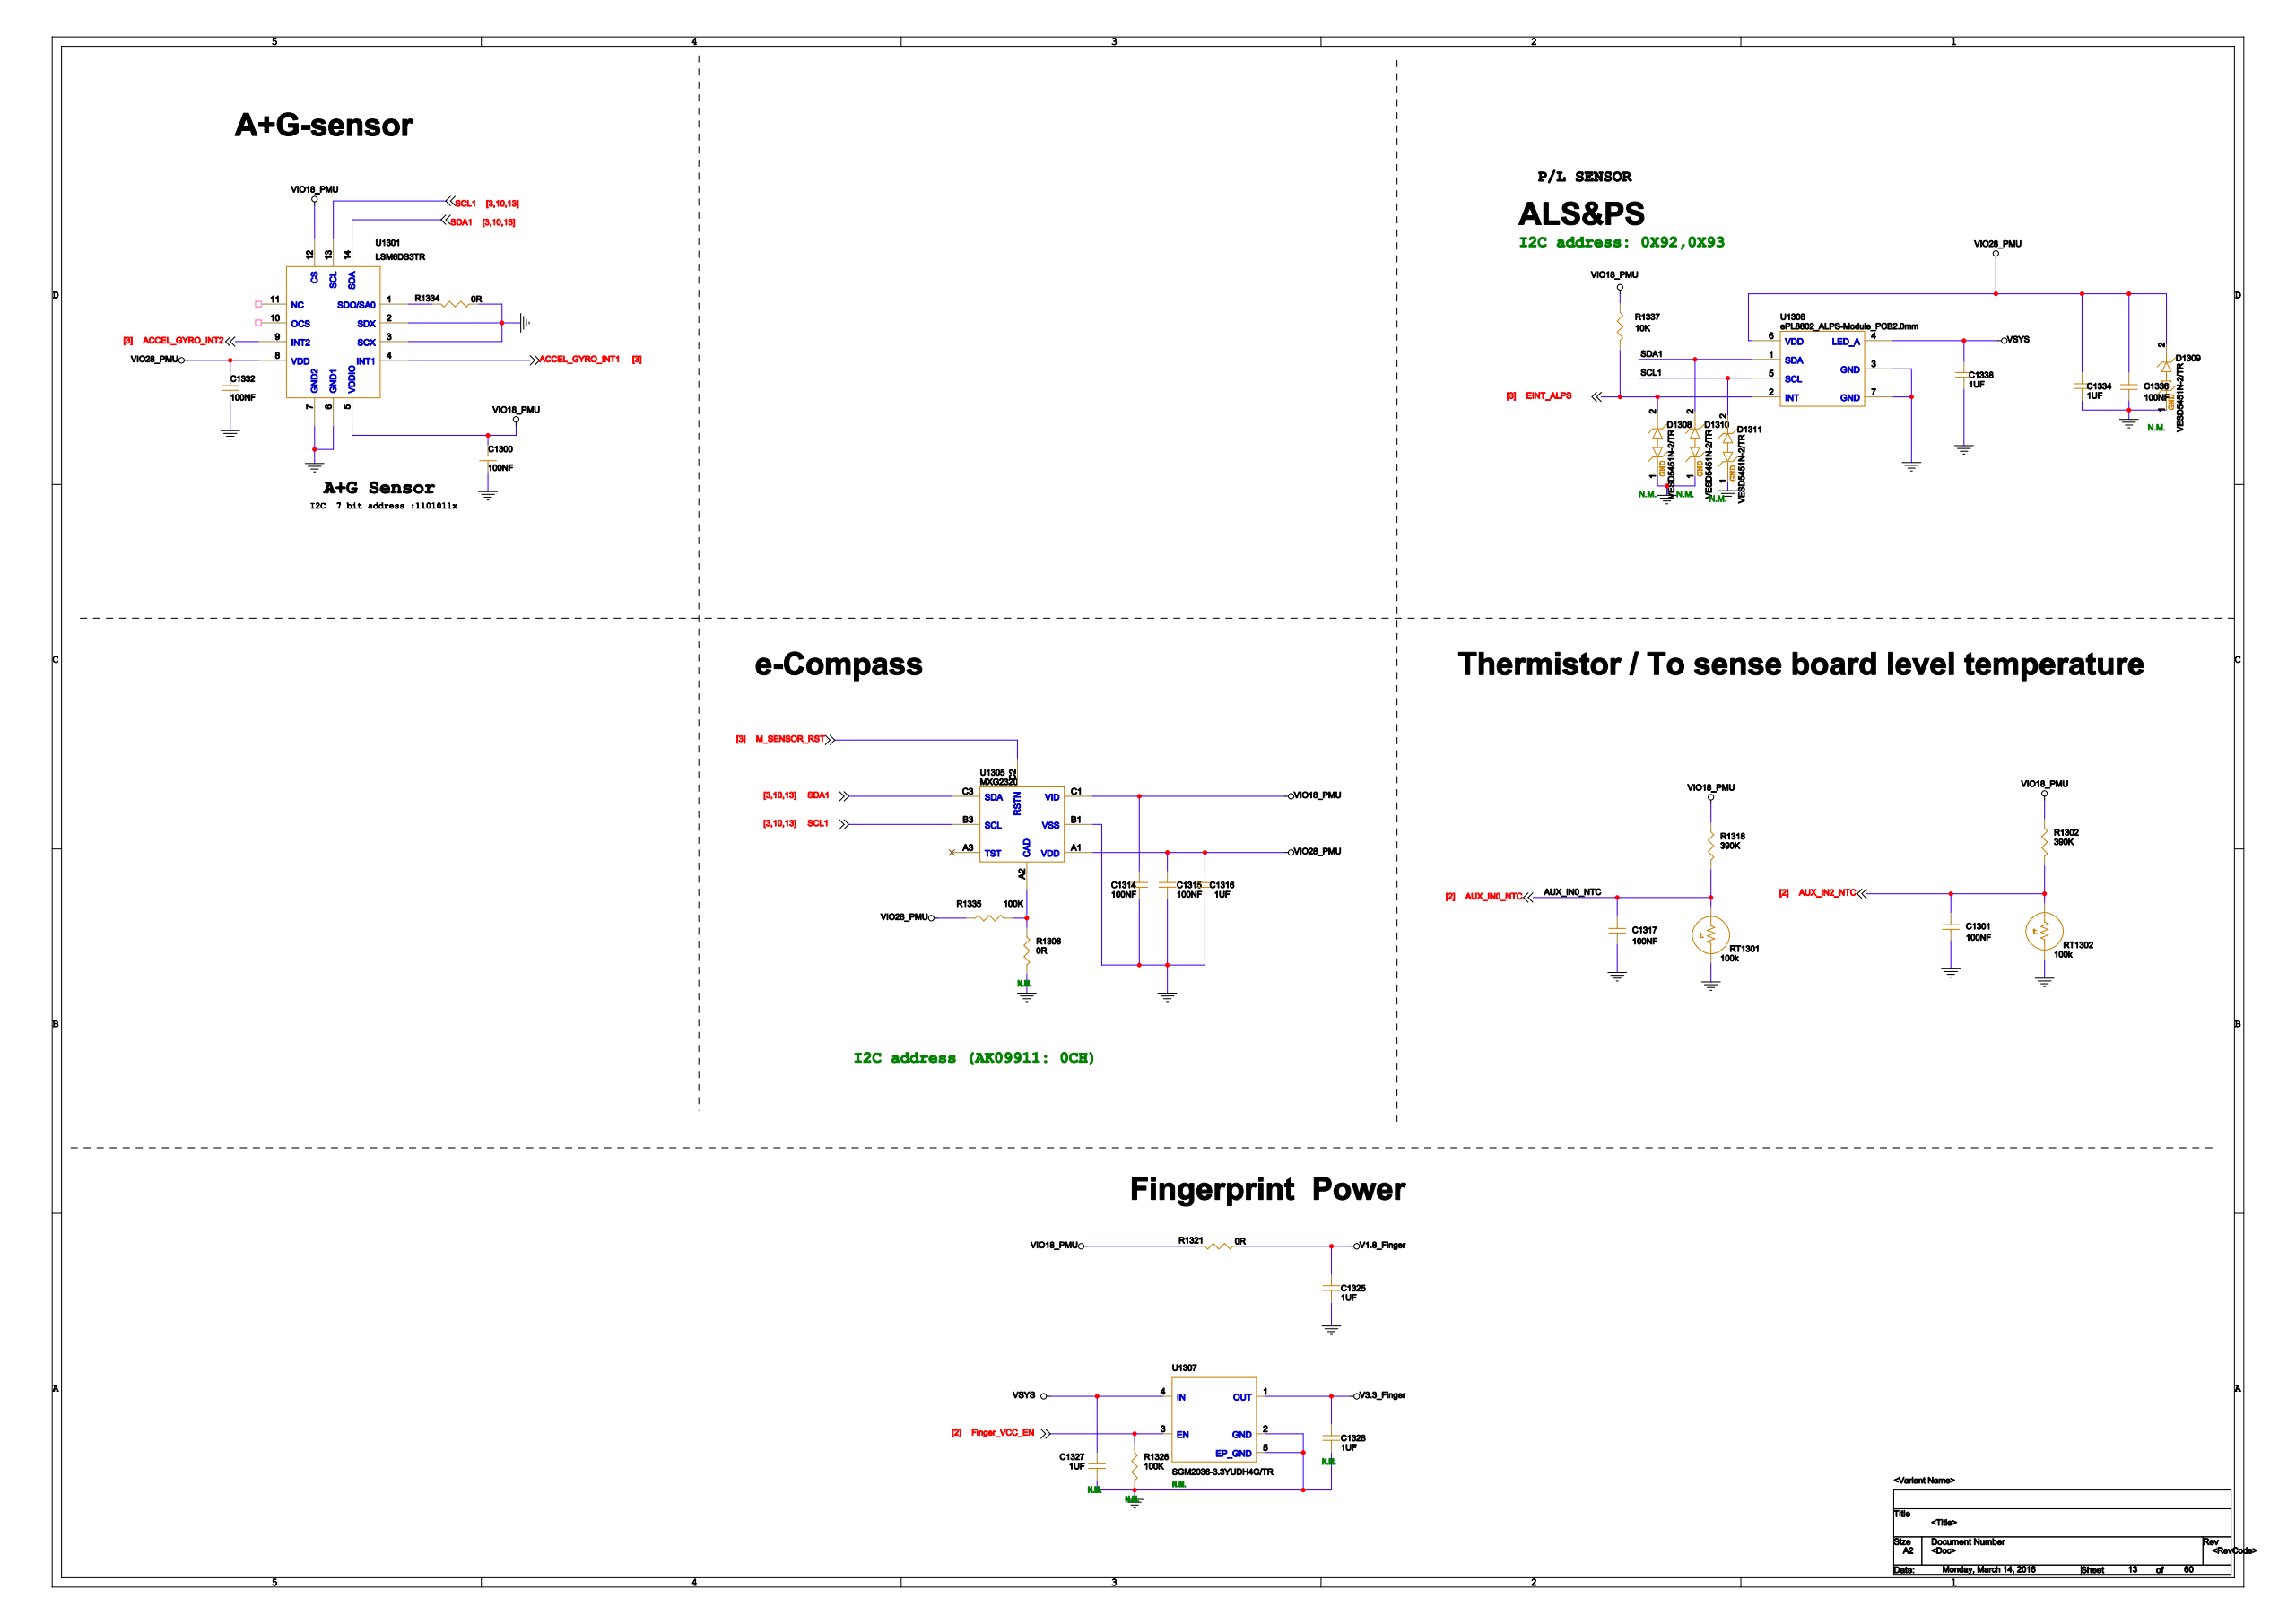Circuit board | Cadence Allegro | 1088 parts | 793 nets | one sheet of the schematic
Parts on this sheet (reference | value | footprint):
C1300 | 100NF | C0201
C1301 | 100NF | C0201
C1314 | 100NF | C0201
C1315 | 100NF | C0201
C1316 | 1UF | C0201
C1317 | 100NF | C0201
C1325 | 1UF | C0201
C1327
C1328
C1332 | 100NF | C0201
C1334 | 1UF | C0201
C1336 | 100NF | C0201
C1338 | 1UF | C0201
D1308
D1309
D1310
D1311
R1302 | 390K | R0201
R1306
R1318 | 390K | R0201
R1321 | 0R | R0201
R1326
R1334 | 0R | R0201
R1335 | 100K | R0201
R1337 | 10K | R0201
RT1301 | 100k | R0201
RT1302 | 100k | R0201
U1301 | LSM6DS3TR | LGA14_2P5X3X0P96_0P5
U1305 | MXG2320 | WLCSP8_1P2X1P2X0P667_0P4
U1307
U1308 | ePL8802_ALPS-Module_PCB2.0mm | EPL8802_ALPS-MODULE_PCB2_0MM
Nets of these parts (net: part-pin ...):
GND: C1300-2 C1301-1 C1314-2 C1315-2 C1316-2 C1317-1 C1325-2 C1327-2 C1328-2 C1332-2 C1334-2 C1336-1 C1338-2 D1308-1 D1309-1 D1310-1 D1311-1 R1306-2 R1326-2 R1334-1 RT1301-2 RT1302-2 U1301-2 U1301-3 U1301-6 U1301-7 U1305-B1 U1307-2 U1307-5 U1308-3 U1308-7
VSYS: C1327-1 C1338-1 U1307-4 U1308-4
EINT_ALPS: D1308-2 R1337-2 U1308-2
SCL1: D1311-2 U1301-13 U1305-B3 U1308-5
SDA1: D1310-2 U1301-14 U1305-C3 U1308-1
VIO28_PMU: C1315-1 C1316-1 C1332-1 C1334-1 C1336-2 D1309-2 R1335-1 U1301-8 U1305-A1 U1308-6
AUX_IN0_NTC: C1317-2 R1318-2 RT1301-1
AUX_IN2_NTC: C1301-2 R1302-2 RT1302-1
ACCEL_GYRO_INT1: U1301-4
ACCEL_GYRO_INT2: U1301-9
FINGER_VCC_EN: R1326-1 U1307-3
M_SENSOR_RST: U1305-C2
VIO18_PMU: C1300-1 C1314-1 R1302-1 R1318-1 R1321-2 R1337-1 U1301-5 U1301-12 U1305-C1
N30718061: R1306-1 R1335-2 U1305-A2
V3.3_FINGER: C1328-1 U1307-1
V1.8_FINGER: C1325-1 R1321-1
N33415412: R1334-2 U1301-1